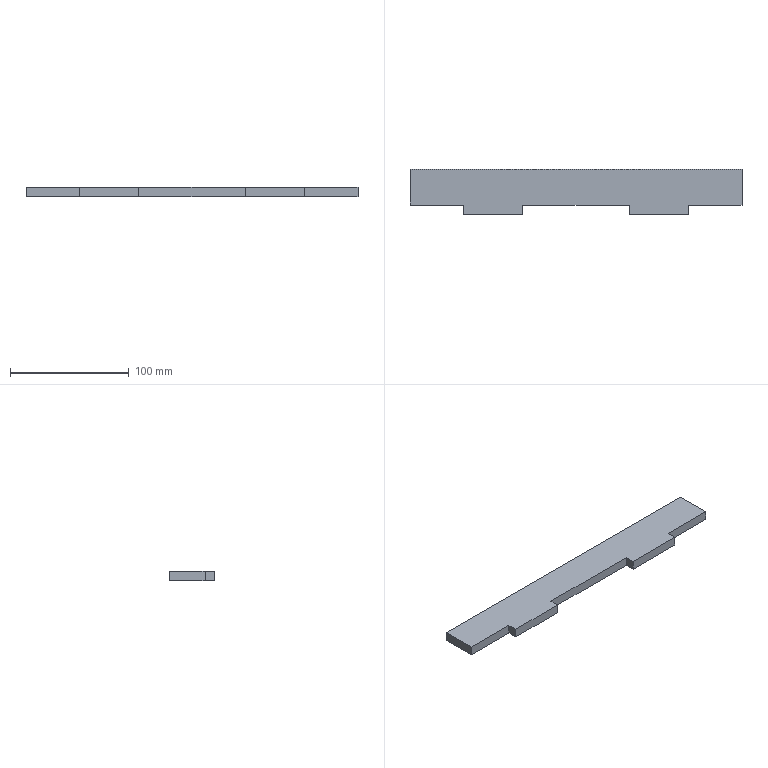Part | SolidWorks | features FlatPattern 1, SMBaseFlange 1, SheetMetal 1 | 1 solid | 14 faces | box 280 x 38 x 8 mm | volume 73600 mm3 | plane 14
STEP:
#1=CARTESIAN_POINT('',(95.,-15.,0.));
#2=VERTEX_POINT('',#1);
#3=CARTESIAN_POINT('',(140.,-15.,0.));
#4=VERTEX_POINT('',#3);
#5=CARTESIAN_POINT('',(95.,-15.,0.));
#6=DIRECTION('',(1.,0.,0.));
#7=VECTOR('',#6,1000.);
#8=LINE('',#5,#7);
#9=EDGE_CURVE('',#2,#4,#8,.T.);
#10=ORIENTED_EDGE('',*,*,#9,.F.);
#11=CARTESIAN_POINT('',(95.,-15.,-8.));
#12=VERTEX_POINT('',#11);
#13=CARTESIAN_POINT('',(95.,-15.,-8.));
#14=DIRECTION('',(0.,0.,1.));
#15=VECTOR('',#14,1000.);
#16=LINE('',#13,#15);
#17=EDGE_CURVE('',#12,#2,#16,.T.);
#18=ORIENTED_EDGE('',*,*,#17,.F.);
#19=CARTESIAN_POINT('',(140.,-15.,-8.));
#20=VERTEX_POINT('',#19);
#21=CARTESIAN_POINT('',(95.,-15.,-8.));
#22=DIRECTION('',(1.,0.,0.));
#23=VECTOR('',#22,1000.);
#24=LINE('',#21,#23);
#25=EDGE_CURVE('',#12,#20,#24,.T.);
#26=ORIENTED_EDGE('',*,*,#25,.T.);
#27=CARTESIAN_POINT('',(140.,-15.,-8.));
#28=DIRECTION('',(0.,0.,1.));
#29=VECTOR('',#28,1000.);
#30=LINE('',#27,#29);
#31=EDGE_CURVE('',#20,#4,#30,.T.);
#32=ORIENTED_EDGE('',*,*,#31,.T.);
#33=EDGE_LOOP('',(#10,#18,#26,#32));
#34=FACE_OUTER_BOUND('',#33,.T.);
#35=CARTESIAN_POINT('',(95.,-15.,-8.));
#36=DIRECTION('',(0.,-1.,0.));
#37=DIRECTION('',(0.,0.,-1.));
#38=AXIS2_PLACEMENT_3D('',#35,#36,#37);
#39=PLANE('',#38);
#40=ADVANCED_FACE('',(#34),#39,.T.);
#41=CARTESIAN_POINT('',(95.,-23.,0.));
#42=VERTEX_POINT('',#41);
#43=CARTESIAN_POINT('',(95.,-15.,0.));
#44=DIRECTION('',(0.,1.,0.));
#45=VECTOR('',#44,1000.);
#46=LINE('',#43,#45);
#47=EDGE_CURVE('',#42,#2,#46,.T.);
#48=ORIENTED_EDGE('',*,*,#47,.F.);
#49=CARTESIAN_POINT('',(95.,-23.,-8.));
#50=VERTEX_POINT('',#49);
#51=CARTESIAN_POINT('',(95.,-23.,-8.));
#52=DIRECTION('',(0.,0.,1.));
#53=VECTOR('',#52,1000.);
#54=LINE('',#51,#53);
#55=EDGE_CURVE('',#50,#42,#54,.T.);
#56=ORIENTED_EDGE('',*,*,#55,.F.);
#57=CARTESIAN_POINT('',(95.,-15.,-8.));
#58=DIRECTION('',(0.,1.,0.));
#59=VECTOR('',#58,1000.);
#60=LINE('',#57,#59);
#61=EDGE_CURVE('',#50,#12,#60,.T.);
#62=ORIENTED_EDGE('',*,*,#61,.T.);
#63=ORIENTED_EDGE('',*,*,#17,.T.);
#64=EDGE_LOOP('',(#48,#56,#62,#63));
#65=FACE_OUTER_BOUND('',#64,.T.);
#66=CARTESIAN_POINT('',(95.,-15.,-8.));
#67=DIRECTION('',(1.,0.,0.));
#68=DIRECTION('',(0.,0.,-1.));
#69=AXIS2_PLACEMENT_3D('',#66,#67,#68);
#70=PLANE('',#69);
#71=ADVANCED_FACE('',(#65),#70,.T.);
#72=CARTESIAN_POINT('',(45.,-23.,0.));
#73=VERTEX_POINT('',#72);
#74=CARTESIAN_POINT('',(45.,-23.,0.));
#75=DIRECTION('',(1.,0.,0.));
#76=VECTOR('',#75,1000.);
#77=LINE('',#74,#76);
#78=EDGE_CURVE('',#73,#42,#77,.T.);
#79=ORIENTED_EDGE('',*,*,#78,.F.);
#80=CARTESIAN_POINT('',(45.,-23.,-8.));
#81=VERTEX_POINT('',#80);
#82=CARTESIAN_POINT('',(45.,-23.,-8.));
#83=DIRECTION('',(0.,0.,1.));
#84=VECTOR('',#83,1000.);
#85=LINE('',#82,#84);
#86=EDGE_CURVE('',#81,#73,#85,.T.);
#87=ORIENTED_EDGE('',*,*,#86,.F.);
#88=CARTESIAN_POINT('',(45.,-23.,-8.));
#89=DIRECTION('',(1.,0.,0.));
#90=VECTOR('',#89,1000.);
#91=LINE('',#88,#90);
#92=EDGE_CURVE('',#81,#50,#91,.T.);
#93=ORIENTED_EDGE('',*,*,#92,.T.);
#94=ORIENTED_EDGE('',*,*,#55,.T.);
#95=EDGE_LOOP('',(#79,#87,#93,#94));
#96=FACE_OUTER_BOUND('',#95,.T.);
#97=CARTESIAN_POINT('',(45.,-23.,-8.));
#98=DIRECTION('',(0.,-1.,0.));
#99=DIRECTION('',(0.,0.,-1.));
#100=AXIS2_PLACEMENT_3D('',#97,#98,#99);
#101=PLANE('',#100);
#102=ADVANCED_FACE('',(#96),#101,.T.);
#103=CARTESIAN_POINT('',(45.,-15.,0.));
#104=VERTEX_POINT('',#103);
#105=CARTESIAN_POINT('',(45.,-23.,0.));
#106=DIRECTION('',(0.,-1.,0.));
#107=VECTOR('',#106,1000.);
#108=LINE('',#105,#107);
#109=EDGE_CURVE('',#104,#73,#108,.T.);
#110=ORIENTED_EDGE('',*,*,#109,.F.);
#111=CARTESIAN_POINT('',(45.,-15.,-8.));
#112=VERTEX_POINT('',#111);
#113=CARTESIAN_POINT('',(45.,-15.,-8.));
#114=DIRECTION('',(0.,0.,1.));
#115=VECTOR('',#114,1000.);
#116=LINE('',#113,#115);
#117=EDGE_CURVE('',#112,#104,#116,.T.);
#118=ORIENTED_EDGE('',*,*,#117,.F.);
#119=CARTESIAN_POINT('',(45.,-23.,-8.));
#120=DIRECTION('',(0.,-1.,0.));
#121=VECTOR('',#120,1000.);
#122=LINE('',#119,#121);
#123=EDGE_CURVE('',#112,#81,#122,.T.);
#124=ORIENTED_EDGE('',*,*,#123,.T.);
#125=ORIENTED_EDGE('',*,*,#86,.T.);
#126=EDGE_LOOP('',(#110,#118,#124,#125));
#127=FACE_OUTER_BOUND('',#126,.T.);
#128=CARTESIAN_POINT('',(45.,-23.,-8.));
#129=DIRECTION('',(-1.,0.,0.));
#130=DIRECTION('',(0.,-1.,0.));
#131=AXIS2_PLACEMENT_3D('',#128,#129,#130);
#132=PLANE('',#131);
#133=ADVANCED_FACE('',(#127),#132,.T.);
#134=CARTESIAN_POINT('',(-45.,-15.,0.));
#135=VERTEX_POINT('',#134);
#136=CARTESIAN_POINT('',(-45.,-15.,0.));
#137=DIRECTION('',(1.,0.,0.));
#138=VECTOR('',#137,1000.);
#139=LINE('',#136,#138);
#140=EDGE_CURVE('',#135,#104,#139,.T.);
#141=ORIENTED_EDGE('',*,*,#140,.F.);
#142=CARTESIAN_POINT('',(-45.,-15.,-8.));
#143=VERTEX_POINT('',#142);
#144=CARTESIAN_POINT('',(-45.,-15.,-8.));
#145=DIRECTION('',(0.,0.,1.));
#146=VECTOR('',#145,1000.);
#147=LINE('',#144,#146);
#148=EDGE_CURVE('',#143,#135,#147,.T.);
#149=ORIENTED_EDGE('',*,*,#148,.F.);
#150=CARTESIAN_POINT('',(-45.,-15.,-8.));
#151=DIRECTION('',(1.,0.,0.));
#152=VECTOR('',#151,1000.);
#153=LINE('',#150,#152);
#154=EDGE_CURVE('',#143,#112,#153,.T.);
#155=ORIENTED_EDGE('',*,*,#154,.T.);
#156=ORIENTED_EDGE('',*,*,#117,.T.);
#157=EDGE_LOOP('',(#141,#149,#155,#156));
#158=FACE_OUTER_BOUND('',#157,.T.);
#159=CARTESIAN_POINT('',(-45.,-15.,-8.));
#160=DIRECTION('',(0.,-1.,0.));
#161=DIRECTION('',(0.,0.,-1.));
#162=AXIS2_PLACEMENT_3D('',#159,#160,#161);
#163=PLANE('',#162);
#164=ADVANCED_FACE('',(#158),#163,.T.);
#165=CARTESIAN_POINT('',(-45.,-23.,0.));
#166=VERTEX_POINT('',#165);
#167=CARTESIAN_POINT('',(-45.,-23.,0.));
#168=DIRECTION('',(0.,1.,0.));
#169=VECTOR('',#168,1000.);
#170=LINE('',#167,#169);
#171=EDGE_CURVE('',#166,#135,#170,.T.);
#172=ORIENTED_EDGE('',*,*,#171,.F.);
#173=CARTESIAN_POINT('',(-45.,-23.,-8.));
#174=VERTEX_POINT('',#173);
#175=CARTESIAN_POINT('',(-45.,-23.,-8.));
#176=DIRECTION('',(0.,0.,1.));
#177=VECTOR('',#176,1000.);
#178=LINE('',#175,#177);
#179=EDGE_CURVE('',#174,#166,#178,.T.);
#180=ORIENTED_EDGE('',*,*,#179,.F.);
#181=CARTESIAN_POINT('',(-45.,-23.,-8.));
#182=DIRECTION('',(0.,1.,0.));
#183=VECTOR('',#182,1000.);
#184=LINE('',#181,#183);
#185=EDGE_CURVE('',#174,#143,#184,.T.);
#186=ORIENTED_EDGE('',*,*,#185,.T.);
#187=ORIENTED_EDGE('',*,*,#148,.T.);
#188=EDGE_LOOP('',(#172,#180,#186,#187));
#189=FACE_OUTER_BOUND('',#188,.T.);
#190=CARTESIAN_POINT('',(-45.,-23.,-8.));
#191=DIRECTION('',(1.,0.,0.));
#192=DIRECTION('',(0.,1.,0.));
#193=AXIS2_PLACEMENT_3D('',#190,#191,#192);
#194=PLANE('',#193);
#195=ADVANCED_FACE('',(#189),#194,.T.);
#196=CARTESIAN_POINT('',(-95.,-23.,0.));
#197=VERTEX_POINT('',#196);
#198=CARTESIAN_POINT('',(-95.,-23.,0.));
#199=DIRECTION('',(1.,0.,0.));
#200=VECTOR('',#199,1000.);
#201=LINE('',#198,#200);
#202=EDGE_CURVE('',#197,#166,#201,.T.);
#203=ORIENTED_EDGE('',*,*,#202,.F.);
#204=CARTESIAN_POINT('',(-95.,-23.,-8.));
#205=VERTEX_POINT('',#204);
#206=CARTESIAN_POINT('',(-95.,-23.,-8.));
#207=DIRECTION('',(0.,0.,1.));
#208=VECTOR('',#207,1000.);
#209=LINE('',#206,#208);
#210=EDGE_CURVE('',#205,#197,#209,.T.);
#211=ORIENTED_EDGE('',*,*,#210,.F.);
#212=CARTESIAN_POINT('',(-95.,-23.,-8.));
#213=DIRECTION('',(1.,0.,0.));
#214=VECTOR('',#213,1000.);
#215=LINE('',#212,#214);
#216=EDGE_CURVE('',#205,#174,#215,.T.);
#217=ORIENTED_EDGE('',*,*,#216,.T.);
#218=ORIENTED_EDGE('',*,*,#179,.T.);
#219=EDGE_LOOP('',(#203,#211,#217,#218));
#220=FACE_OUTER_BOUND('',#219,.T.);
#221=CARTESIAN_POINT('',(-95.,-23.,-8.));
#222=DIRECTION('',(0.,-1.,0.));
#223=DIRECTION('',(0.,0.,-1.));
#224=AXIS2_PLACEMENT_3D('',#221,#222,#223);
#225=PLANE('',#224);
#226=ADVANCED_FACE('',(#220),#225,.T.);
#227=CARTESIAN_POINT('',(-95.,-15.,0.));
#228=VERTEX_POINT('',#227);
#229=CARTESIAN_POINT('',(-95.,-15.,0.));
#230=DIRECTION('',(0.,-1.,0.));
#231=VECTOR('',#230,1000.);
#232=LINE('',#229,#231);
#233=EDGE_CURVE('',#228,#197,#232,.T.);
#234=ORIENTED_EDGE('',*,*,#233,.F.);
#235=CARTESIAN_POINT('',(-95.,-15.,-8.));
#236=VERTEX_POINT('',#235);
#237=CARTESIAN_POINT('',(-95.,-15.,-8.));
#238=DIRECTION('',(0.,0.,1.));
#239=VECTOR('',#238,1000.);
#240=LINE('',#237,#239);
#241=EDGE_CURVE('',#236,#228,#240,.T.);
#242=ORIENTED_EDGE('',*,*,#241,.F.);
#243=CARTESIAN_POINT('',(-95.,-15.,-8.));
#244=DIRECTION('',(0.,-1.,0.));
#245=VECTOR('',#244,1000.);
#246=LINE('',#243,#245);
#247=EDGE_CURVE('',#236,#205,#246,.T.);
#248=ORIENTED_EDGE('',*,*,#247,.T.);
#249=ORIENTED_EDGE('',*,*,#210,.T.);
#250=EDGE_LOOP('',(#234,#242,#248,#249));
#251=FACE_OUTER_BOUND('',#250,.T.);
#252=CARTESIAN_POINT('',(-95.,-15.,-8.));
#253=DIRECTION('',(-1.,0.,0.));
#254=DIRECTION('',(0.,0.,1.));
#255=AXIS2_PLACEMENT_3D('',#252,#253,#254);
#256=PLANE('',#255);
#257=ADVANCED_FACE('',(#251),#256,.T.);
#258=CARTESIAN_POINT('',(-140.,-15.,0.));
#259=VERTEX_POINT('',#258);
#260=CARTESIAN_POINT('',(-140.,-15.,0.));
#261=DIRECTION('',(1.,0.,0.));
#262=VECTOR('',#261,1000.);
#263=LINE('',#260,#262);
#264=EDGE_CURVE('',#259,#228,#263,.T.);
#265=ORIENTED_EDGE('',*,*,#264,.F.);
#266=CARTESIAN_POINT('',(-140.,-15.,-8.));
#267=VERTEX_POINT('',#266);
#268=CARTESIAN_POINT('',(-140.,-15.,-8.));
#269=DIRECTION('',(0.,0.,1.));
#270=VECTOR('',#269,1000.);
#271=LINE('',#268,#270);
#272=EDGE_CURVE('',#267,#259,#271,.T.);
#273=ORIENTED_EDGE('',*,*,#272,.F.);
#274=CARTESIAN_POINT('',(-140.,-15.,-8.));
#275=DIRECTION('',(1.,0.,0.));
#276=VECTOR('',#275,1000.);
#277=LINE('',#274,#276);
#278=EDGE_CURVE('',#267,#236,#277,.T.);
#279=ORIENTED_EDGE('',*,*,#278,.T.);
#280=ORIENTED_EDGE('',*,*,#241,.T.);
#281=EDGE_LOOP('',(#265,#273,#279,#280));
#282=FACE_OUTER_BOUND('',#281,.T.);
#283=CARTESIAN_POINT('',(-140.,-15.,-8.));
#284=DIRECTION('',(0.,-1.,0.));
#285=DIRECTION('',(0.,0.,-1.));
#286=AXIS2_PLACEMENT_3D('',#283,#284,#285);
#287=PLANE('',#286);
#288=ADVANCED_FACE('',(#282),#287,.T.);
#289=CARTESIAN_POINT('',(-140.,15.,0.));
#290=VERTEX_POINT('',#289);
#291=CARTESIAN_POINT('',(-140.,15.,0.));
#292=DIRECTION('',(0.,-1.,0.));
#293=VECTOR('',#292,1000.);
#294=LINE('',#291,#293);
#295=EDGE_CURVE('',#290,#259,#294,.T.);
#296=ORIENTED_EDGE('',*,*,#295,.F.);
#297=CARTESIAN_POINT('',(-140.,15.,-8.));
#298=VERTEX_POINT('',#297);
#299=CARTESIAN_POINT('',(-140.,15.,-8.));
#300=DIRECTION('',(0.,0.,1.));
#301=VECTOR('',#300,1000.);
#302=LINE('',#299,#301);
#303=EDGE_CURVE('',#298,#290,#302,.T.);
#304=ORIENTED_EDGE('',*,*,#303,.F.);
#305=CARTESIAN_POINT('',(-140.,15.,-8.));
#306=DIRECTION('',(0.,-1.,0.));
#307=VECTOR('',#306,1000.);
#308=LINE('',#305,#307);
#309=EDGE_CURVE('',#298,#267,#308,.T.);
#310=ORIENTED_EDGE('',*,*,#309,.T.);
#311=ORIENTED_EDGE('',*,*,#272,.T.);
#312=EDGE_LOOP('',(#296,#304,#310,#311));
#313=FACE_OUTER_BOUND('',#312,.T.);
#314=CARTESIAN_POINT('',(-140.,15.,-8.));
#315=DIRECTION('',(-1.,0.,0.));
#316=DIRECTION('',(0.,0.,1.));
#317=AXIS2_PLACEMENT_3D('',#314,#315,#316);
#318=PLANE('',#317);
#319=ADVANCED_FACE('',(#313),#318,.T.);
#320=CARTESIAN_POINT('',(140.,15.,0.));
#321=VERTEX_POINT('',#320);
#322=CARTESIAN_POINT('',(-140.,15.,0.));
#323=DIRECTION('',(-1.,0.,0.));
#324=VECTOR('',#323,1000.);
#325=LINE('',#322,#324);
#326=EDGE_CURVE('',#321,#290,#325,.T.);
#327=ORIENTED_EDGE('',*,*,#326,.F.);
#328=CARTESIAN_POINT('',(140.,15.,-8.));
#329=VERTEX_POINT('',#328);
#330=CARTESIAN_POINT('',(140.,15.,-8.));
#331=DIRECTION('',(0.,0.,1.));
#332=VECTOR('',#331,1000.);
#333=LINE('',#330,#332);
#334=EDGE_CURVE('',#329,#321,#333,.T.);
#335=ORIENTED_EDGE('',*,*,#334,.F.);
#336=CARTESIAN_POINT('',(-140.,15.,-8.));
#337=DIRECTION('',(-1.,0.,0.));
#338=VECTOR('',#337,1000.);
#339=LINE('',#336,#338);
#340=EDGE_CURVE('',#329,#298,#339,.T.);
#341=ORIENTED_EDGE('',*,*,#340,.T.);
#342=ORIENTED_EDGE('',*,*,#303,.T.);
#343=EDGE_LOOP('',(#327,#335,#341,#342));
#344=FACE_OUTER_BOUND('',#343,.T.);
#345=CARTESIAN_POINT('',(-140.,15.,-8.));
#346=DIRECTION('',(0.,1.,0.));
#347=DIRECTION('',(0.,0.,1.));
#348=AXIS2_PLACEMENT_3D('',#345,#346,#347);
#349=PLANE('',#348);
#350=ADVANCED_FACE('',(#344),#349,.T.);
#351=CARTESIAN_POINT('',(140.,15.,0.));
#352=DIRECTION('',(0.,1.,0.));
#353=VECTOR('',#352,1000.);
#354=LINE('',#351,#353);
#355=EDGE_CURVE('',#4,#321,#354,.T.);
#356=ORIENTED_EDGE('',*,*,#355,.F.);
#357=ORIENTED_EDGE('',*,*,#31,.F.);
#358=CARTESIAN_POINT('',(140.,15.,-8.));
#359=DIRECTION('',(0.,1.,0.));
#360=VECTOR('',#359,1000.);
#361=LINE('',#358,#360);
#362=EDGE_CURVE('',#20,#329,#361,.T.);
#363=ORIENTED_EDGE('',*,*,#362,.T.);
#364=ORIENTED_EDGE('',*,*,#334,.T.);
#365=EDGE_LOOP('',(#356,#357,#363,#364));
#366=FACE_OUTER_BOUND('',#365,.T.);
#367=CARTESIAN_POINT('',(140.,15.,-8.));
#368=DIRECTION('',(1.,0.,0.));
#369=DIRECTION('',(0.,0.,-1.));
#370=AXIS2_PLACEMENT_3D('',#367,#368,#369);
#371=PLANE('',#370);
#372=ADVANCED_FACE('',(#366),#371,.T.);
#373=ORIENTED_EDGE('',*,*,#25,.F.);
#374=ORIENTED_EDGE('',*,*,#61,.F.);
#375=ORIENTED_EDGE('',*,*,#92,.F.);
#376=ORIENTED_EDGE('',*,*,#123,.F.);
#377=ORIENTED_EDGE('',*,*,#154,.F.);
#378=ORIENTED_EDGE('',*,*,#185,.F.);
#379=ORIENTED_EDGE('',*,*,#216,.F.);
#380=ORIENTED_EDGE('',*,*,#247,.F.);
#381=ORIENTED_EDGE('',*,*,#278,.F.);
#382=ORIENTED_EDGE('',*,*,#309,.F.);
#383=ORIENTED_EDGE('',*,*,#340,.F.);
#384=ORIENTED_EDGE('',*,*,#362,.F.);
#385=EDGE_LOOP('',(#373,#374,#375,#376,#377,#378,#379,#380,#381,#382,#383,#384));
#386=FACE_OUTER_BOUND('',#385,.T.);
#387=CARTESIAN_POINT('',(0.,0.,-8.));
#388=DIRECTION('',(0.,0.,-1.));
#389=DIRECTION('',(-1.,0.,0.));
#390=AXIS2_PLACEMENT_3D('',#387,#388,#389);
#391=PLANE('',#390);
#392=ADVANCED_FACE('',(#386),#391,.T.);
#393=ORIENTED_EDGE('',*,*,#9,.T.);
#394=ORIENTED_EDGE('',*,*,#355,.T.);
#395=ORIENTED_EDGE('',*,*,#326,.T.);
#396=ORIENTED_EDGE('',*,*,#295,.T.);
#397=ORIENTED_EDGE('',*,*,#264,.T.);
#398=ORIENTED_EDGE('',*,*,#233,.T.);
#399=ORIENTED_EDGE('',*,*,#202,.T.);
#400=ORIENTED_EDGE('',*,*,#171,.T.);
#401=ORIENTED_EDGE('',*,*,#140,.T.);
#402=ORIENTED_EDGE('',*,*,#109,.T.);
#403=ORIENTED_EDGE('',*,*,#78,.T.);
#404=ORIENTED_EDGE('',*,*,#47,.T.);
#405=EDGE_LOOP('',(#393,#394,#395,#396,#397,#398,#399,#400,#401,#402,#403,#404));
#406=FACE_OUTER_BOUND('',#405,.T.);
#407=CARTESIAN_POINT('',(0.,0.,0.));
#408=DIRECTION('',(0.,0.,-1.));
#409=DIRECTION('',(-1.,0.,0.));
#410=AXIS2_PLACEMENT_3D('',#407,#408,#409);
#411=PLANE('',#410);
#412=ADVANCED_FACE('',(#406),#411,.F.);
#413=CLOSED_SHELL('',(#40,#71,#102,#133,#164,#195,#226,#257,#288,#319,#350,#372,#392,#412));
#414=MANIFOLD_SOLID_BREP('',#413);
#415=CARTESIAN_POINT('',(0.,0.,0.));
#416=DIRECTION('',(0.,0.,1.));
#417=DIRECTION('',(1.,0.,0.));
#418=AXIS2_PLACEMENT_3D('',#415,#416,#417);
#419=(LENGTH_UNIT()NAMED_UNIT(*)SI_UNIT(.MILLI.,.METRE.));
#420=UNCERTAINTY_MEASURE_WITH_UNIT(LENGTH_MEASURE(0.00001),#419,'','');
#421=(NAMED_UNIT(*)PLANE_ANGLE_UNIT()SI_UNIT($,.RADIAN.));
#422=(NAMED_UNIT(*)SI_UNIT($,.STERADIAN.)SOLID_ANGLE_UNIT());
#423=(GEOMETRIC_REPRESENTATION_CONTEXT(3)GLOBAL_UNCERTAINTY_ASSIGNED_CONTEXT((#420))GLOBAL_UNIT_ASSIGNED_CONTEXT((#419,#421,#422))REPRESENTATION_CONTEXT('',''));
#424=ADVANCED_BREP_SHAPE_REPRESENTATION('',(#414,#418),#423);